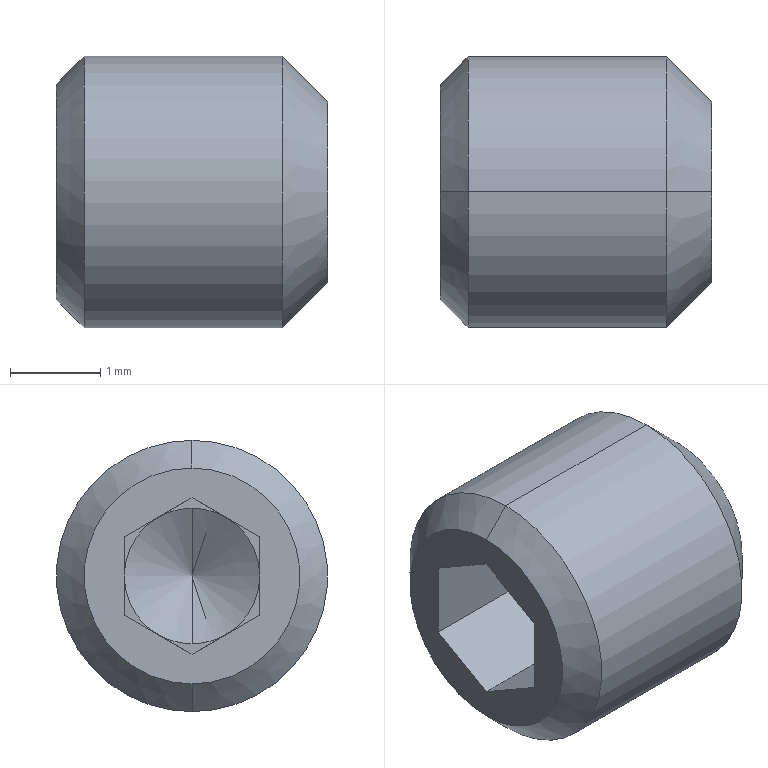Part | SolidWorks | features BaseBody 1 | 1 solid | 22 faces | box 3 x 3 x 3 mm | volume 17.153 mm3 | plane 14 | cone 6 | cylinder 2 | commonest cylinder face diameters 3 x2
STEP:
#1=CARTESIAN_POINT('',(-3.,0.,-1.194));
#2=VERTEX_POINT('',#1);
#3=CARTESIAN_POINT('',(-3.,0.,1.194));
#4=VERTEX_POINT('',#3);
#5=CARTESIAN_POINT('',(-3.,0.,0.));
#6=DIRECTION('',(1.,0.,0.));
#7=DIRECTION('',(0.,0.,-1.));
#8=AXIS2_PLACEMENT_3D('',#5,#6,#7);
#9=CIRCLE('',#8,1.194);
#10=EDGE_CURVE('',#2,#4,#9,.T.);
#11=ORIENTED_EDGE('',*,*,#10,.T.);
#12=CARTESIAN_POINT('',(-2.694,0.,1.5));
#13=VERTEX_POINT('',#12);
#14=CARTESIAN_POINT('',(-3.,0.,1.194));
#15=DIRECTION('',(0.7071,0.,0.7071));
#16=VECTOR('',#15,1000.);
#17=LINE('',#14,#16);
#18=EDGE_CURVE('',#4,#13,#17,.T.);
#19=ORIENTED_EDGE('',*,*,#18,.T.);
#20=CARTESIAN_POINT('',(-2.694,0.,-1.5));
#21=VERTEX_POINT('',#20);
#22=CARTESIAN_POINT('',(-2.694,0.,0.));
#23=DIRECTION('',(1.,0.,0.));
#24=DIRECTION('',(0.,0.,-1.));
#25=AXIS2_PLACEMENT_3D('',#22,#23,#24);
#26=CIRCLE('',#25,1.5);
#27=EDGE_CURVE('',#21,#13,#26,.T.);
#28=ORIENTED_EDGE('',*,*,#27,.F.);
#29=CARTESIAN_POINT('',(-3.,0.,-1.194));
#30=DIRECTION('',(0.7071,0.,-0.7071));
#31=VECTOR('',#30,1000.);
#32=LINE('',#29,#31);
#33=EDGE_CURVE('',#2,#21,#32,.T.);
#34=ORIENTED_EDGE('',*,*,#33,.F.);
#35=EDGE_LOOP('',(#11,#19,#28,#34));
#36=FACE_OUTER_BOUND('',#35,.T.);
#37=CARTESIAN_POINT('',(-3.,0.,0.));
#38=DIRECTION('',(1.,0.,0.));
#39=DIRECTION('',(0.,0.,-1.));
#40=AXIS2_PLACEMENT_3D('',#37,#38,#39);
#41=CONICAL_SURFACE('',#40,1.194,0.7854);
#42=ADVANCED_FACE('',(#36),#41,.T.);
#43=ORIENTED_EDGE('',*,*,#27,.T.);
#44=CARTESIAN_POINT('',(-0.5,0.,1.5));
#45=VERTEX_POINT('',#44);
#46=CARTESIAN_POINT('',(0.,0.,1.5));
#47=DIRECTION('',(1.,0.,0.));
#48=VECTOR('',#47,1000.);
#49=LINE('',#46,#48);
#50=EDGE_CURVE('',#13,#45,#49,.T.);
#51=ORIENTED_EDGE('',*,*,#50,.T.);
#52=CARTESIAN_POINT('',(-0.5,0.,-1.5));
#53=VERTEX_POINT('',#52);
#54=CARTESIAN_POINT('',(-0.5,0.,0.));
#55=DIRECTION('',(1.,0.,0.));
#56=DIRECTION('',(0.,0.,-1.));
#57=AXIS2_PLACEMENT_3D('',#54,#55,#56);
#58=CIRCLE('',#57,1.5);
#59=EDGE_CURVE('',#53,#45,#58,.T.);
#60=ORIENTED_EDGE('',*,*,#59,.F.);
#61=CARTESIAN_POINT('',(0.,0.,-1.5));
#62=DIRECTION('',(1.,0.,0.));
#63=VECTOR('',#62,1000.);
#64=LINE('',#61,#63);
#65=EDGE_CURVE('',#21,#53,#64,.T.);
#66=ORIENTED_EDGE('',*,*,#65,.F.);
#67=EDGE_LOOP('',(#43,#51,#60,#66));
#68=FACE_OUTER_BOUND('',#67,.T.);
#69=CARTESIAN_POINT('',(0.,0.,0.));
#70=DIRECTION('',(1.,0.,0.));
#71=DIRECTION('',(0.,0.,-1.));
#72=AXIS2_PLACEMENT_3D('',#69,#70,#71);
#73=CYLINDRICAL_SURFACE('',#72,1.5);
#74=ADVANCED_FACE('',(#68),#73,.T.);
#75=CARTESIAN_POINT('',(0.,0.,-1.));
#76=VERTEX_POINT('',#75);
#77=CARTESIAN_POINT('',(0.,0.,1.));
#78=VERTEX_POINT('',#77);
#79=CARTESIAN_POINT('',(0.,0.,0.));
#80=DIRECTION('',(1.,0.,0.));
#81=DIRECTION('',(0.,0.,-1.));
#82=AXIS2_PLACEMENT_3D('',#79,#80,#81);
#83=CIRCLE('',#82,1.);
#84=EDGE_CURVE('',#76,#78,#83,.T.);
#85=ORIENTED_EDGE('',*,*,#84,.F.);
#86=CARTESIAN_POINT('',(-0.5,0.,-1.5));
#87=DIRECTION('',(-0.7071,0.,-0.7071));
#88=VECTOR('',#87,1000.);
#89=LINE('',#86,#88);
#90=EDGE_CURVE('',#76,#53,#89,.T.);
#91=ORIENTED_EDGE('',*,*,#90,.T.);
#92=ORIENTED_EDGE('',*,*,#59,.T.);
#93=CARTESIAN_POINT('',(-0.5,0.,1.5));
#94=DIRECTION('',(-0.7071,0.,0.7071));
#95=VECTOR('',#94,1000.);
#96=LINE('',#93,#95);
#97=EDGE_CURVE('',#78,#45,#96,.T.);
#98=ORIENTED_EDGE('',*,*,#97,.F.);
#99=EDGE_LOOP('',(#85,#91,#92,#98));
#100=FACE_OUTER_BOUND('',#99,.T.);
#101=CARTESIAN_POINT('',(-0.5,0.,0.));
#102=DIRECTION('',(-1.,0.,0.));
#103=DIRECTION('',(0.,0.,1.));
#104=AXIS2_PLACEMENT_3D('',#101,#102,#103);
#105=CONICAL_SURFACE('',#104,1.5,0.7854);
#106=ADVANCED_FACE('',(#100),#105,.T.);
#107=CARTESIAN_POINT('',(-1.367,0.,0.));
#108=VERTEX_POINT('',#107);
#109=CARTESIAN_POINT('',(-1.8,0.,0.75));
#110=VERTEX_POINT('',#109);
#111=CARTESIAN_POINT('',(-1.8,0.,0.75));
#112=DIRECTION('',(-0.5,0.,0.866));
#113=VECTOR('',#112,1000.);
#114=LINE('',#111,#113);
#115=EDGE_CURVE('',#108,#110,#114,.T.);
#116=ORIENTED_EDGE('',*,*,#115,.F.);
#117=CARTESIAN_POINT('',(-1.8,0.,-0.75));
#118=VERTEX_POINT('',#117);
#119=CARTESIAN_POINT('',(-1.8,0.,-0.75));
#120=DIRECTION('',(-0.5,0.,-0.866));
#121=VECTOR('',#120,1000.);
#122=LINE('',#119,#121);
#123=EDGE_CURVE('',#108,#118,#122,.T.);
#124=ORIENTED_EDGE('',*,*,#123,.T.);
#125=CARTESIAN_POINT('',(-1.8,-0.375,-0.6495));
#126=VERTEX_POINT('',#125);
#127=CARTESIAN_POINT('',(-1.8,0.,0.));
#128=DIRECTION('',(1.,0.,0.));
#129=DIRECTION('',(0.,0.,1.));
#130=AXIS2_PLACEMENT_3D('',#127,#128,#129);
#131=CIRCLE('',#130,0.75);
#132=EDGE_CURVE('',#126,#118,#131,.T.);
#133=ORIENTED_EDGE('',*,*,#132,.F.);
#134=CARTESIAN_POINT('',(-1.8,-0.75,0.));
#135=VERTEX_POINT('',#134);
#136=CARTESIAN_POINT('',(-1.8,0.,0.));
#137=DIRECTION('',(1.,0.,0.));
#138=DIRECTION('',(0.,0.,1.));
#139=AXIS2_PLACEMENT_3D('',#136,#137,#138);
#140=CIRCLE('',#139,0.75);
#141=EDGE_CURVE('',#135,#126,#140,.T.);
#142=ORIENTED_EDGE('',*,*,#141,.F.);
#143=CARTESIAN_POINT('',(-1.8,-0.375,0.6495));
#144=VERTEX_POINT('',#143);
#145=CARTESIAN_POINT('',(-1.8,0.,0.));
#146=DIRECTION('',(1.,0.,0.));
#147=DIRECTION('',(0.,0.,1.));
#148=AXIS2_PLACEMENT_3D('',#145,#146,#147);
#149=CIRCLE('',#148,0.75);
#150=EDGE_CURVE('',#144,#135,#149,.T.);
#151=ORIENTED_EDGE('',*,*,#150,.F.);
#152=CARTESIAN_POINT('',(-1.8,0.,0.));
#153=DIRECTION('',(1.,0.,0.));
#154=DIRECTION('',(0.,0.,1.));
#155=AXIS2_PLACEMENT_3D('',#152,#153,#154);
#156=CIRCLE('',#155,0.75);
#157=EDGE_CURVE('',#110,#144,#156,.T.);
#158=ORIENTED_EDGE('',*,*,#157,.F.);
#159=EDGE_LOOP('',(#116,#124,#133,#142,#151,#158));
#160=FACE_OUTER_BOUND('',#159,.T.);
#161=CARTESIAN_POINT('',(-1.8,0.,0.));
#162=DIRECTION('',(-1.,0.,0.));
#163=DIRECTION('',(0.,0.,1.));
#164=AXIS2_PLACEMENT_3D('',#161,#162,#163);
#165=CONICAL_SURFACE('',#164,0.75,1.047);
#166=ADVANCED_FACE('',(#160),#165,.F.);
#167=ORIENTED_EDGE('',*,*,#123,.F.);
#168=ORIENTED_EDGE('',*,*,#115,.T.);
#169=CARTESIAN_POINT('',(-1.8,0.375,0.6495));
#170=VERTEX_POINT('',#169);
#171=CARTESIAN_POINT('',(-1.8,0.,0.));
#172=DIRECTION('',(1.,0.,0.));
#173=DIRECTION('',(0.,0.,1.));
#174=AXIS2_PLACEMENT_3D('',#171,#172,#173);
#175=CIRCLE('',#174,0.75);
#176=EDGE_CURVE('',#170,#110,#175,.T.);
#177=ORIENTED_EDGE('',*,*,#176,.F.);
#178=CARTESIAN_POINT('',(-1.8,0.75,0.));
#179=VERTEX_POINT('',#178);
#180=CARTESIAN_POINT('',(-1.8,0.,0.));
#181=DIRECTION('',(1.,0.,0.));
#182=DIRECTION('',(0.,0.,-1.));
#183=AXIS2_PLACEMENT_3D('',#180,#181,#182);
#184=CIRCLE('',#183,0.75);
#185=EDGE_CURVE('',#179,#170,#184,.T.);
#186=ORIENTED_EDGE('',*,*,#185,.F.);
#187=CARTESIAN_POINT('',(-1.8,0.375,-0.6495));
#188=VERTEX_POINT('',#187);
#189=CARTESIAN_POINT('',(-1.8,0.,0.));
#190=DIRECTION('',(1.,0.,0.));
#191=DIRECTION('',(0.,0.,1.));
#192=AXIS2_PLACEMENT_3D('',#189,#190,#191);
#193=CIRCLE('',#192,0.75);
#194=EDGE_CURVE('',#188,#179,#193,.T.);
#195=ORIENTED_EDGE('',*,*,#194,.F.);
#196=CARTESIAN_POINT('',(-1.8,0.,0.));
#197=DIRECTION('',(1.,0.,0.));
#198=DIRECTION('',(0.,0.,1.));
#199=AXIS2_PLACEMENT_3D('',#196,#197,#198);
#200=CIRCLE('',#199,0.75);
#201=EDGE_CURVE('',#118,#188,#200,.T.);
#202=ORIENTED_EDGE('',*,*,#201,.F.);
#203=EDGE_LOOP('',(#167,#168,#177,#186,#195,#202));
#204=FACE_OUTER_BOUND('',#203,.T.);
#205=CARTESIAN_POINT('',(-1.8,0.,0.));
#206=DIRECTION('',(-1.,0.,0.));
#207=DIRECTION('',(0.,0.,1.));
#208=AXIS2_PLACEMENT_3D('',#205,#206,#207);
#209=CONICAL_SURFACE('',#208,0.75,1.047);
#210=ADVANCED_FACE('',(#204),#209,.F.);
#211=CARTESIAN_POINT('',(-1.8,0.,0.866));
#212=VERTEX_POINT('',#211);
#213=CARTESIAN_POINT('',(-1.8,0.,0.866));
#214=DIRECTION('',(0.,0.866,-0.5));
#215=VECTOR('',#214,1000.);
#216=LINE('',#213,#215);
#217=EDGE_CURVE('',#212,#170,#216,.T.);
#218=ORIENTED_EDGE('',*,*,#217,.T.);
#219=ORIENTED_EDGE('',*,*,#176,.T.);
#220=ORIENTED_EDGE('',*,*,#157,.T.);
#221=CARTESIAN_POINT('',(-1.8,-0.75,0.433));
#222=DIRECTION('',(0.,0.866,0.5));
#223=VECTOR('',#222,1000.);
#224=LINE('',#221,#223);
#225=EDGE_CURVE('',#144,#212,#224,.T.);
#226=ORIENTED_EDGE('',*,*,#225,.T.);
#227=EDGE_LOOP('',(#218,#219,#220,#226));
#228=FACE_OUTER_BOUND('',#227,.T.);
#229=CARTESIAN_POINT('',(-1.8,0.,0.));
#230=DIRECTION('',(-1.,0.,0.));
#231=DIRECTION('',(0.,0.,1.));
#232=AXIS2_PLACEMENT_3D('',#229,#230,#231);
#233=PLANE('',#232);
#234=ADVANCED_FACE('',(#228),#233,.T.);
#235=CARTESIAN_POINT('',(-3.,0.,-0.866));
#236=VERTEX_POINT('',#235);
#237=CARTESIAN_POINT('',(-3.,-0.75,-0.433));
#238=VERTEX_POINT('',#237);
#239=CARTESIAN_POINT('',(-3.,0.,-0.866));
#240=DIRECTION('',(0.,-0.866,0.5));
#241=VECTOR('',#240,1000.);
#242=LINE('',#239,#241);
#243=EDGE_CURVE('',#236,#238,#242,.T.);
#244=ORIENTED_EDGE('',*,*,#243,.T.);
#245=CARTESIAN_POINT('',(-1.8,-0.75,-0.433));
#246=VERTEX_POINT('',#245);
#247=CARTESIAN_POINT('',(-1.8,-0.75,-0.433));
#248=DIRECTION('',(-1.,0.,0.));
#249=VECTOR('',#248,1000.);
#250=LINE('',#247,#249);
#251=EDGE_CURVE('',#246,#238,#250,.T.);
#252=ORIENTED_EDGE('',*,*,#251,.F.);
#253=CARTESIAN_POINT('',(-1.8,0.,-0.866));
#254=DIRECTION('',(0.,-0.866,0.5));
#255=VECTOR('',#254,1000.);
#256=LINE('',#253,#255);
#257=EDGE_CURVE('',#126,#246,#256,.T.);
#258=ORIENTED_EDGE('',*,*,#257,.F.);
#259=CARTESIAN_POINT('',(-1.8,0.,-0.866));
#260=VERTEX_POINT('',#259);
#261=CARTESIAN_POINT('',(-1.8,0.,-0.866));
#262=DIRECTION('',(0.,-0.866,0.5));
#263=VECTOR('',#262,1000.);
#264=LINE('',#261,#263);
#265=EDGE_CURVE('',#260,#126,#264,.T.);
#266=ORIENTED_EDGE('',*,*,#265,.F.);
#267=CARTESIAN_POINT('',(-1.8,0.,-0.866));
#268=DIRECTION('',(-1.,0.,0.));
#269=VECTOR('',#268,1000.);
#270=LINE('',#267,#269);
#271=EDGE_CURVE('',#260,#236,#270,.T.);
#272=ORIENTED_EDGE('',*,*,#271,.T.);
#273=EDGE_LOOP('',(#244,#252,#258,#266,#272));
#274=FACE_OUTER_BOUND('',#273,.T.);
#275=CARTESIAN_POINT('',(-1.8,0.,-0.866));
#276=DIRECTION('',(0.,-0.5,-0.866));
#277=DIRECTION('',(0.,-0.866,0.5));
#278=AXIS2_PLACEMENT_3D('',#275,#276,#277);
#279=PLANE('',#278);
#280=ADVANCED_FACE('',(#274),#279,.F.);
#281=CARTESIAN_POINT('',(-3.,0.75,-0.433));
#282=VERTEX_POINT('',#281);
#283=CARTESIAN_POINT('',(-3.,0.75,-0.433));
#284=DIRECTION('',(0.,-0.866,-0.5));
#285=VECTOR('',#284,1000.);
#286=LINE('',#283,#285);
#287=EDGE_CURVE('',#282,#236,#286,.T.);
#288=ORIENTED_EDGE('',*,*,#287,.T.);
#289=ORIENTED_EDGE('',*,*,#271,.F.);
#290=CARTESIAN_POINT('',(-1.8,0.75,-0.433));
#291=DIRECTION('',(0.,-0.866,-0.5));
#292=VECTOR('',#291,1000.);
#293=LINE('',#290,#292);
#294=EDGE_CURVE('',#188,#260,#293,.T.);
#295=ORIENTED_EDGE('',*,*,#294,.F.);
#296=CARTESIAN_POINT('',(-1.8,0.75,-0.433));
#297=VERTEX_POINT('',#296);
#298=CARTESIAN_POINT('',(-1.8,0.75,-0.433));
#299=DIRECTION('',(0.,-0.866,-0.5));
#300=VECTOR('',#299,1000.);
#301=LINE('',#298,#300);
#302=EDGE_CURVE('',#297,#188,#301,.T.);
#303=ORIENTED_EDGE('',*,*,#302,.F.);
#304=CARTESIAN_POINT('',(-1.8,0.75,-0.433));
#305=DIRECTION('',(-1.,0.,0.));
#306=VECTOR('',#305,1000.);
#307=LINE('',#304,#306);
#308=EDGE_CURVE('',#297,#282,#307,.T.);
#309=ORIENTED_EDGE('',*,*,#308,.T.);
#310=EDGE_LOOP('',(#288,#289,#295,#303,#309));
#311=FACE_OUTER_BOUND('',#310,.T.);
#312=CARTESIAN_POINT('',(-1.8,0.75,-0.433));
#313=DIRECTION('',(0.,0.5,-0.866));
#314=DIRECTION('',(-1.,0.,0.));
#315=AXIS2_PLACEMENT_3D('',#312,#313,#314);
#316=PLANE('',#315);
#317=ADVANCED_FACE('',(#311),#316,.F.);
#318=CARTESIAN_POINT('',(-1.8,0.75,0.433));
#319=VERTEX_POINT('',#318);
#320=CARTESIAN_POINT('',(-3.,0.75,0.433));
#321=VERTEX_POINT('',#320);
#322=CARTESIAN_POINT('',(-1.8,0.75,0.433));
#323=DIRECTION('',(-1.,0.,0.));
#324=VECTOR('',#323,1000.);
#325=LINE('',#322,#324);
#326=EDGE_CURVE('',#319,#321,#325,.T.);
#327=ORIENTED_EDGE('',*,*,#326,.T.);
#328=CARTESIAN_POINT('',(-3.,0.75,0.));
#329=DIRECTION('',(0.,0.,1.));
#330=VECTOR('',#329,1000.);
#331=LINE('',#328,#330);
#332=EDGE_CURVE('',#282,#321,#331,.T.);
#333=ORIENTED_EDGE('',*,*,#332,.F.);
#334=ORIENTED_EDGE('',*,*,#308,.F.);
#335=CARTESIAN_POINT('',(-1.8,0.75,0.433));
#336=DIRECTION('',(0.,0.,-1.));
#337=VECTOR('',#336,1000.);
#338=LINE('',#335,#337);
#339=EDGE_CURVE('',#179,#297,#338,.T.);
#340=ORIENTED_EDGE('',*,*,#339,.F.);
#341=CARTESIAN_POINT('',(-1.8,0.75,0.433));
#342=DIRECTION('',(0.,0.,-1.));
#343=VECTOR('',#342,1000.);
#344=LINE('',#341,#343);
#345=EDGE_CURVE('',#319,#179,#344,.T.);
#346=ORIENTED_EDGE('',*,*,#345,.F.);
#347=EDGE_LOOP('',(#327,#333,#334,#340,#346));
#348=FACE_OUTER_BOUND('',#347,.T.);
#349=CARTESIAN_POINT('',(-1.8,0.75,0.433));
#350=DIRECTION('',(0.,1.,0.));
#351=DIRECTION('',(1.,0.,0.));
#352=AXIS2_PLACEMENT_3D('',#349,#350,#351);
#353=PLANE('',#352);
#354=ADVANCED_FACE('',(#348),#353,.F.);
#355=CARTESIAN_POINT('',(-3.,0.,0.866));
#356=VERTEX_POINT('',#355);
#357=CARTESIAN_POINT('',(-3.,0.,0.866));
#358=DIRECTION('',(0.,0.866,-0.5));
#359=VECTOR('',#358,1000.);
#360=LINE('',#357,#359);
#361=EDGE_CURVE('',#356,#321,#360,.T.);
#362=ORIENTED_EDGE('',*,*,#361,.T.);
#363=ORIENTED_EDGE('',*,*,#326,.F.);
#364=CARTESIAN_POINT('',(-1.8,0.,0.866));
#365=DIRECTION('',(0.,0.866,-0.5));
#366=VECTOR('',#365,1000.);
#367=LINE('',#364,#366);
#368=EDGE_CURVE('',#170,#319,#367,.T.);
#369=ORIENTED_EDGE('',*,*,#368,.F.);
#370=ORIENTED_EDGE('',*,*,#217,.F.);
#371=CARTESIAN_POINT('',(-1.8,0.,0.866));
#372=DIRECTION('',(-1.,0.,0.));
#373=VECTOR('',#372,1000.);
#374=LINE('',#371,#373);
#375=EDGE_CURVE('',#212,#356,#374,.T.);
#376=ORIENTED_EDGE('',*,*,#375,.T.);
#377=EDGE_LOOP('',(#362,#363,#369,#370,#376));
#378=FACE_OUTER_BOUND('',#377,.T.);
#379=CARTESIAN_POINT('',(-1.8,0.,0.866));
#380=DIRECTION('',(0.,0.5,0.866));
#381=DIRECTION('',(1.,0.,0.));
#382=AXIS2_PLACEMENT_3D('',#379,#380,#381);
#383=PLANE('',#382);
#384=ADVANCED_FACE('',(#378),#383,.F.);
#385=CARTESIAN_POINT('',(-3.,-0.75,0.433));
#386=VERTEX_POINT('',#385);
#387=CARTESIAN_POINT('',(-3.,-0.75,0.433));
#388=DIRECTION('',(0.,0.866,0.5));
#389=VECTOR('',#388,1000.);
#390=LINE('',#387,#389);
#391=EDGE_CURVE('',#386,#356,#390,.T.);
#392=ORIENTED_EDGE('',*,*,#391,.T.);
#393=ORIENTED_EDGE('',*,*,#375,.F.);
#394=ORIENTED_EDGE('',*,*,#225,.F.);
#395=CARTESIAN_POINT('',(-1.8,-0.75,0.433));
#396=VERTEX_POINT('',#395);
#397=CARTESIAN_POINT('',(-1.8,-0.75,0.433));
#398=DIRECTION('',(0.,0.866,0.5));
#399=VECTOR('',#398,1000.);
#400=LINE('',#397,#399);
#401=EDGE_CURVE('',#396,#144,#400,.T.);
#402=ORIENTED_EDGE('',*,*,#401,.F.);
#403=CARTESIAN_POINT('',(-1.8,-0.75,0.433));
#404=DIRECTION('',(-1.,0.,0.));
#405=VECTOR('',#404,1000.);
#406=LINE('',#403,#405);
#407=EDGE_CURVE('',#396,#386,#406,.T.);
#408=ORIENTED_EDGE('',*,*,#407,.T.);
#409=EDGE_LOOP('',(#392,#393,#394,#402,#408));
#410=FACE_OUTER_BOUND('',#409,.T.);
#411=CARTESIAN_POINT('',(-1.8,-0.75,0.433));
#412=DIRECTION('',(0.,-0.5,0.866));
#413=DIRECTION('',(-1.,0.,0.));
#414=AXIS2_PLACEMENT_3D('',#411,#412,#413);
#415=PLANE('',#414);
#416=ADVANCED_FACE('',(#410),#415,.F.);
#417=CARTESIAN_POINT('',(-3.,-0.75,-0.433));
#418=DIRECTION('',(0.,0.,1.));
#419=VECTOR('',#418,1000.);
#420=LINE('',#417,#419);
#421=EDGE_CURVE('',#238,#386,#420,.T.);
#422=ORIENTED_EDGE('',*,*,#421,.T.);
#423=ORIENTED_EDGE('',*,*,#407,.F.);
#424=CARTESIAN_POINT('',(-1.8,-0.75,-0.433));
#425=DIRECTION('',(0.,0.,1.));
#426=VECTOR('',#425,1000.);
#427=LINE('',#424,#426);
#428=EDGE_CURVE('',#135,#396,#427,.T.);
#429=ORIENTED_EDGE('',*,*,#428,.F.);
#430=CARTESIAN_POINT('',(-1.8,-0.75,-0.433));
#431=DIRECTION('',(0.,0.,1.));
#432=VECTOR('',#431,1000.);
#433=LINE('',#430,#432);
#434=EDGE_CURVE('',#246,#135,#433,.T.);
#435=ORIENTED_EDGE('',*,*,#434,.F.);
#436=ORIENTED_EDGE('',*,*,#251,.T.);
#437=EDGE_LOOP('',(#422,#423,#429,#435,#436));
#438=FACE_OUTER_BOUND('',#437,.T.);
#439=CARTESIAN_POINT('',(-1.8,-0.75,-0.433));
#440=DIRECTION('',(0.,-1.,0.));
#441=DIRECTION('',(0.,0.,-1.));
#442=AXIS2_PLACEMENT_3D('',#439,#440,#441);
#443=PLANE('',#442);
#444=ADVANCED_FACE('',(#438),#443,.F.);
#445=CARTESIAN_POINT('',(0.,0.,0.));
#446=DIRECTION('',(1.,0.,0.));
#447=DIRECTION('',(0.,0.,-1.));
#448=AXIS2_PLACEMENT_3D('',#445,#446,#447);
#449=CIRCLE('',#448,1.);
#450=EDGE_CURVE('',#78,#76,#449,.T.);
#451=ORIENTED_EDGE('',*,*,#450,.T.);
#452=ORIENTED_EDGE('',*,*,#84,.T.);
#453=EDGE_LOOP('',(#451,#452));
#454=FACE_OUTER_BOUND('',#453,.T.);
#455=CARTESIAN_POINT('',(0.,1.,0.));
#456=DIRECTION('',(-1.,0.,0.));
#457=DIRECTION('',(0.,0.,1.));
#458=AXIS2_PLACEMENT_3D('',#455,#456,#457);
#459=PLANE('',#458);
#460=ADVANCED_FACE('',(#454),#459,.F.);
#461=ORIENTED_EDGE('',*,*,#90,.F.);
#462=ORIENTED_EDGE('',*,*,#450,.F.);
#463=ORIENTED_EDGE('',*,*,#97,.T.);
#464=CARTESIAN_POINT('',(-0.5,0.,0.));
#465=DIRECTION('',(1.,0.,0.));
#466=DIRECTION('',(0.,0.,-1.));
#467=AXIS2_PLACEMENT_3D('',#464,#465,#466);
#468=CIRCLE('',#467,1.5);
#469=EDGE_CURVE('',#45,#53,#468,.T.);
#470=ORIENTED_EDGE('',*,*,#469,.T.);
#471=EDGE_LOOP('',(#461,#462,#463,#470));
#472=FACE_OUTER_BOUND('',#471,.T.);
#473=CARTESIAN_POINT('',(-0.5,0.,0.));
#474=DIRECTION('',(-1.,0.,0.));
#475=DIRECTION('',(0.,0.,1.));
#476=AXIS2_PLACEMENT_3D('',#473,#474,#475);
#477=CONICAL_SURFACE('',#476,1.5,0.7854);
#478=ADVANCED_FACE('',(#472),#477,.T.);
#479=ORIENTED_EDGE('',*,*,#50,.F.);
#480=CARTESIAN_POINT('',(-2.694,0.,0.));
#481=DIRECTION('',(1.,0.,0.));
#482=DIRECTION('',(0.,0.,-1.));
#483=AXIS2_PLACEMENT_3D('',#480,#481,#482);
#484=CIRCLE('',#483,1.5);
#485=EDGE_CURVE('',#13,#21,#484,.T.);
#486=ORIENTED_EDGE('',*,*,#485,.T.);
#487=ORIENTED_EDGE('',*,*,#65,.T.);
#488=ORIENTED_EDGE('',*,*,#469,.F.);
#489=EDGE_LOOP('',(#479,#486,#487,#488));
#490=FACE_OUTER_BOUND('',#489,.T.);
#491=CARTESIAN_POINT('',(0.,0.,0.));
#492=DIRECTION('',(1.,0.,0.));
#493=DIRECTION('',(0.,0.,-1.));
#494=AXIS2_PLACEMENT_3D('',#491,#492,#493);
#495=CYLINDRICAL_SURFACE('',#494,1.5);
#496=ADVANCED_FACE('',(#490),#495,.T.);
#497=ORIENTED_EDGE('',*,*,#18,.F.);
#498=CARTESIAN_POINT('',(-3.,0.,0.));
#499=DIRECTION('',(1.,0.,0.));
#500=DIRECTION('',(0.,0.,-1.));
#501=AXIS2_PLACEMENT_3D('',#498,#499,#500);
#502=CIRCLE('',#501,1.194);
#503=EDGE_CURVE('',#4,#2,#502,.T.);
#504=ORIENTED_EDGE('',*,*,#503,.T.);
#505=ORIENTED_EDGE('',*,*,#33,.T.);
#506=ORIENTED_EDGE('',*,*,#485,.F.);
#507=EDGE_LOOP('',(#497,#504,#505,#506));
#508=FACE_OUTER_BOUND('',#507,.T.);
#509=CARTESIAN_POINT('',(-3.,0.,0.));
#510=DIRECTION('',(1.,0.,0.));
#511=DIRECTION('',(0.,0.,-1.));
#512=AXIS2_PLACEMENT_3D('',#509,#510,#511);
#513=CONICAL_SURFACE('',#512,1.194,0.7854);
#514=ADVANCED_FACE('',(#508),#513,.T.);
#515=ORIENTED_EDGE('',*,*,#361,.F.);
#516=ORIENTED_EDGE('',*,*,#391,.F.);
#517=ORIENTED_EDGE('',*,*,#421,.F.);
#518=ORIENTED_EDGE('',*,*,#243,.F.);
#519=ORIENTED_EDGE('',*,*,#287,.F.);
#520=ORIENTED_EDGE('',*,*,#332,.T.);
#521=EDGE_LOOP('',(#515,#516,#517,#518,#519,#520));
#522=FACE_BOUND('',#521,.T.);
#523=ORIENTED_EDGE('',*,*,#10,.F.);
#524=ORIENTED_EDGE('',*,*,#503,.F.);
#525=EDGE_LOOP('',(#523,#524));
#526=FACE_OUTER_BOUND('',#525,.T.);
#527=CARTESIAN_POINT('',(-3.,0.,0.));
#528=DIRECTION('',(1.,0.,0.));
#529=DIRECTION('',(0.,1.,0.));
#530=AXIS2_PLACEMENT_3D('',#527,#528,#529);
#531=PLANE('',#530);
#532=ADVANCED_FACE('',(#522,#526),#531,.F.);
#533=ORIENTED_EDGE('',*,*,#345,.T.);
#534=ORIENTED_EDGE('',*,*,#185,.T.);
#535=ORIENTED_EDGE('',*,*,#368,.T.);
#536=EDGE_LOOP('',(#533,#534,#535));
#537=FACE_OUTER_BOUND('',#536,.T.);
#538=CARTESIAN_POINT('',(-1.8,0.,0.));
#539=DIRECTION('',(-1.,0.,0.));
#540=DIRECTION('',(0.,0.,1.));
#541=AXIS2_PLACEMENT_3D('',#538,#539,#540);
#542=PLANE('',#541);
#543=ADVANCED_FACE('',(#537),#542,.T.);
#544=ORIENTED_EDGE('',*,*,#302,.T.);
#545=ORIENTED_EDGE('',*,*,#194,.T.);
#546=ORIENTED_EDGE('',*,*,#339,.T.);
#547=EDGE_LOOP('',(#544,#545,#546));
#548=FACE_OUTER_BOUND('',#547,.T.);
#549=CARTESIAN_POINT('',(-1.8,0.,0.));
#550=DIRECTION('',(-1.,0.,0.));
#551=DIRECTION('',(0.,0.,1.));
#552=AXIS2_PLACEMENT_3D('',#549,#550,#551);
#553=PLANE('',#552);
#554=ADVANCED_FACE('',(#548),#553,.T.);
#555=ORIENTED_EDGE('',*,*,#265,.T.);
#556=ORIENTED_EDGE('',*,*,#132,.T.);
#557=ORIENTED_EDGE('',*,*,#201,.T.);
#558=ORIENTED_EDGE('',*,*,#294,.T.);
#559=EDGE_LOOP('',(#555,#556,#557,#558));
#560=FACE_OUTER_BOUND('',#559,.T.);
#561=CARTESIAN_POINT('',(-1.8,0.,0.));
#562=DIRECTION('',(-1.,0.,0.));
#563=DIRECTION('',(0.,0.,1.));
#564=AXIS2_PLACEMENT_3D('',#561,#562,#563);
#565=PLANE('',#564);
#566=ADVANCED_FACE('',(#560),#565,.T.);
#567=ORIENTED_EDGE('',*,*,#434,.T.);
#568=ORIENTED_EDGE('',*,*,#141,.T.);
#569=ORIENTED_EDGE('',*,*,#257,.T.);
#570=EDGE_LOOP('',(#567,#568,#569));
#571=FACE_OUTER_BOUND('',#570,.T.);
#572=CARTESIAN_POINT('',(-1.8,0.,0.));
#573=DIRECTION('',(-1.,0.,0.));
#574=DIRECTION('',(0.,0.,1.));
#575=AXIS2_PLACEMENT_3D('',#572,#573,#574);
#576=PLANE('',#575);
#577=ADVANCED_FACE('',(#571),#576,.T.);
#578=ORIENTED_EDGE('',*,*,#401,.T.);
#579=ORIENTED_EDGE('',*,*,#150,.T.);
#580=ORIENTED_EDGE('',*,*,#428,.T.);
#581=EDGE_LOOP('',(#578,#579,#580));
#582=FACE_OUTER_BOUND('',#581,.T.);
#583=CARTESIAN_POINT('',(-1.8,0.,0.));
#584=DIRECTION('',(-1.,0.,0.));
#585=DIRECTION('',(0.,0.,1.));
#586=AXIS2_PLACEMENT_3D('',#583,#584,#585);
#587=PLANE('',#586);
#588=ADVANCED_FACE('',(#582),#587,.T.);
#589=CLOSED_SHELL('',(#42,#74,#106,#166,#210,#234,#280,#317,#354,#384,#416,#444,#460,#478,#496,#514,#532,#543,#554,#566,#577,#588));
#590=MANIFOLD_SOLID_BREP('',#589);
#591=CARTESIAN_POINT('',(0.,0.,0.));
#592=DIRECTION('',(0.,0.,1.));
#593=DIRECTION('',(1.,0.,0.));
#594=AXIS2_PLACEMENT_3D('',#591,#592,#593);
#595=(LENGTH_UNIT()NAMED_UNIT(*)SI_UNIT(.MILLI.,.METRE.));
#596=UNCERTAINTY_MEASURE_WITH_UNIT(LENGTH_MEASURE(0.00001),#595,'','');
#597=(NAMED_UNIT(*)PLANE_ANGLE_UNIT()SI_UNIT($,.RADIAN.));
#598=(NAMED_UNIT(*)SI_UNIT($,.STERADIAN.)SOLID_ANGLE_UNIT());
#599=(GEOMETRIC_REPRESENTATION_CONTEXT(3)GLOBAL_UNCERTAINTY_ASSIGNED_CONTEXT((#596))GLOBAL_UNIT_ASSIGNED_CONTEXT((#595,#597,#598))REPRESENTATION_CONTEXT('',''));
#600=ADVANCED_BREP_SHAPE_REPRESENTATION('',(#590,#594),#599);